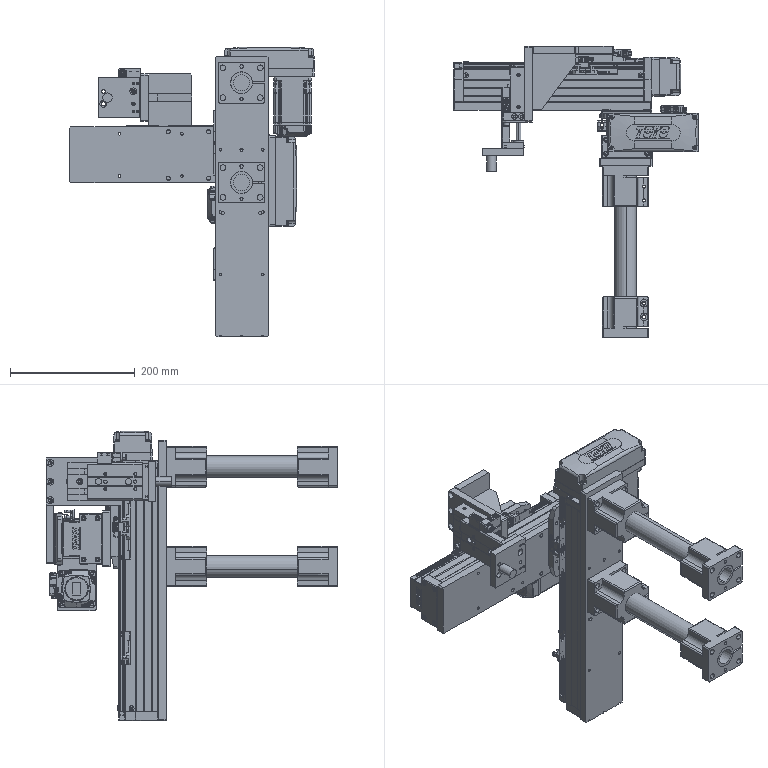Part | SolidWorks | 50 solids | 10611 faces | volume 7253169 mm3 | plane 5094 | cylinder 3174 | spline 1556 | cone 667 | torus 120 | commonest cylinder face diameters 0.4 x318 4 x299 0.6 x236 1 x226 2 x194 5.5 x114